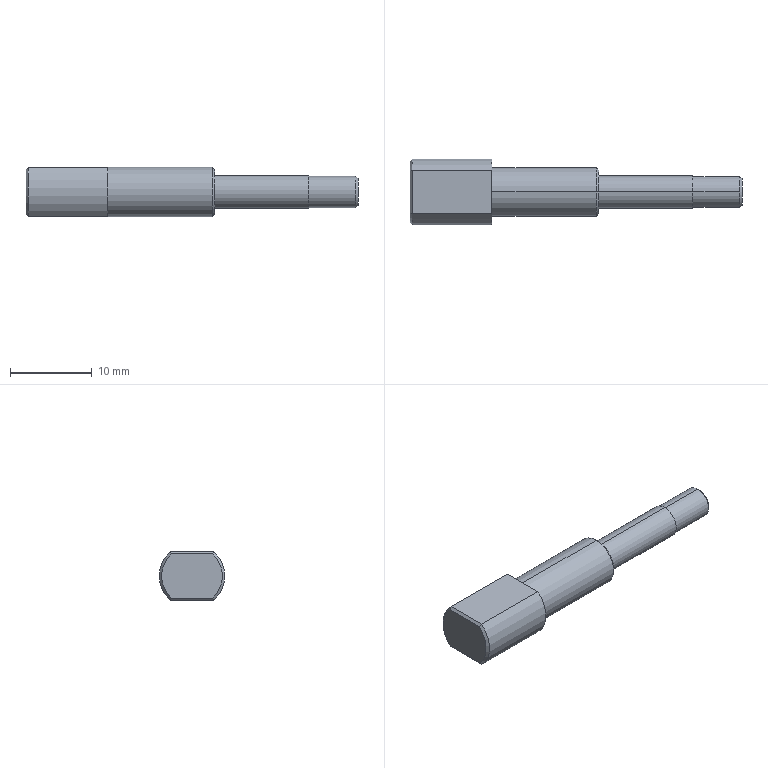Part | SolidWorks | features Chamfer 1, ICE 1, Revolution 1 | 1 solid | 24 faces | box 40.5 x 8 x 6 mm | volume 1008 mm3 | plane 10 | cylinder 8 | cone 6 | commonest cylinder face diameters 3.8 x2 4 x2 6 x2 8 x2
STEP:
#1=CARTESIAN_POINT('',(23.,0.,-2.7));
#2=VERTEX_POINT('',#1);
#3=CARTESIAN_POINT('',(23.,0.,2.7));
#4=VERTEX_POINT('',#3);
#5=CARTESIAN_POINT('',(23.,0.,0.));
#6=DIRECTION('',(1.,0.,0.));
#7=DIRECTION('',(0.,0.,1.));
#8=AXIS2_PLACEMENT_3D('',#5,#6,#7);
#9=CIRCLE('',#8,2.7);
#10=EDGE_CURVE('',#2,#4,#9,.T.);
#11=ORIENTED_EDGE('',*,*,#10,.F.);
#12=CARTESIAN_POINT('',(22.7,0.,-3.));
#13=VERTEX_POINT('',#12);
#14=CARTESIAN_POINT('',(22.7,0.,-3.));
#15=DIRECTION('',(-0.7071,0.,-0.7071));
#16=VECTOR('',#15,1000.);
#17=LINE('',#14,#16);
#18=EDGE_CURVE('',#2,#13,#17,.T.);
#19=ORIENTED_EDGE('',*,*,#18,.T.);
#20=CARTESIAN_POINT('',(22.7,0.,3.));
#21=VERTEX_POINT('',#20);
#22=CARTESIAN_POINT('',(22.7,0.,0.));
#23=DIRECTION('',(-1.,0.,0.));
#24=DIRECTION('',(0.,0.,1.));
#25=AXIS2_PLACEMENT_3D('',#22,#23,#24);
#26=CIRCLE('',#25,3.);
#27=EDGE_CURVE('',#21,#13,#26,.T.);
#28=ORIENTED_EDGE('',*,*,#27,.F.);
#29=CARTESIAN_POINT('',(22.7,0.,3.));
#30=DIRECTION('',(-0.7071,0.,0.7071));
#31=VECTOR('',#30,1000.);
#32=LINE('',#29,#31);
#33=EDGE_CURVE('',#4,#21,#32,.T.);
#34=ORIENTED_EDGE('',*,*,#33,.F.);
#35=EDGE_LOOP('',(#11,#19,#28,#34));
#36=FACE_OUTER_BOUND('',#35,.T.);
#37=CARTESIAN_POINT('',(22.7,0.,0.));
#38=DIRECTION('',(-1.,0.,0.));
#39=DIRECTION('',(0.,0.,1.));
#40=AXIS2_PLACEMENT_3D('',#37,#38,#39);
#41=CONICAL_SURFACE('',#40,3.,0.7854);
#42=ADVANCED_FACE('',(#36),#41,.T.);
#43=CARTESIAN_POINT('',(40.5,0.,-1.6));
#44=VERTEX_POINT('',#43);
#45=CARTESIAN_POINT('',(40.5,0.,1.6));
#46=VERTEX_POINT('',#45);
#47=CARTESIAN_POINT('',(40.5,0.,0.));
#48=DIRECTION('',(1.,0.,0.));
#49=DIRECTION('',(0.,0.,1.));
#50=AXIS2_PLACEMENT_3D('',#47,#48,#49);
#51=CIRCLE('',#50,1.6);
#52=EDGE_CURVE('',#44,#46,#51,.T.);
#53=ORIENTED_EDGE('',*,*,#52,.F.);
#54=CARTESIAN_POINT('',(40.2,0.,-1.9));
#55=VERTEX_POINT('',#54);
#56=CARTESIAN_POINT('',(40.2,0.,-1.9));
#57=DIRECTION('',(-0.7071,0.,-0.7071));
#58=VECTOR('',#57,1000.);
#59=LINE('',#56,#58);
#60=EDGE_CURVE('',#44,#55,#59,.T.);
#61=ORIENTED_EDGE('',*,*,#60,.T.);
#62=CARTESIAN_POINT('',(40.2,0.,1.9));
#63=VERTEX_POINT('',#62);
#64=CARTESIAN_POINT('',(40.2,0.,0.));
#65=DIRECTION('',(-1.,0.,0.));
#66=DIRECTION('',(0.,0.,1.));
#67=AXIS2_PLACEMENT_3D('',#64,#65,#66);
#68=CIRCLE('',#67,1.9);
#69=EDGE_CURVE('',#63,#55,#68,.T.);
#70=ORIENTED_EDGE('',*,*,#69,.F.);
#71=CARTESIAN_POINT('',(40.2,0.,1.9));
#72=DIRECTION('',(-0.7071,0.,0.7071));
#73=VECTOR('',#72,1000.);
#74=LINE('',#71,#73);
#75=EDGE_CURVE('',#46,#63,#74,.T.);
#76=ORIENTED_EDGE('',*,*,#75,.F.);
#77=EDGE_LOOP('',(#53,#61,#70,#76));
#78=FACE_OUTER_BOUND('',#77,.T.);
#79=CARTESIAN_POINT('',(40.2,0.,0.));
#80=DIRECTION('',(-1.,0.,0.));
#81=DIRECTION('',(0.,0.,1.));
#82=AXIS2_PLACEMENT_3D('',#79,#80,#81);
#83=CONICAL_SURFACE('',#82,1.9,0.7854);
#84=ADVANCED_FACE('',(#78),#83,.T.);
#85=ORIENTED_EDGE('',*,*,#69,.T.);
#86=CARTESIAN_POINT('',(34.5,0.,-1.9));
#87=VERTEX_POINT('',#86);
#88=CARTESIAN_POINT('',(0.,0.,-1.9));
#89=DIRECTION('',(-1.,0.,0.));
#90=VECTOR('',#89,1000.);
#91=LINE('',#88,#90);
#92=EDGE_CURVE('',#55,#87,#91,.T.);
#93=ORIENTED_EDGE('',*,*,#92,.T.);
#94=CARTESIAN_POINT('',(34.5,0.,1.9));
#95=VERTEX_POINT('',#94);
#96=CARTESIAN_POINT('',(34.5,0.,0.));
#97=DIRECTION('',(-1.,0.,0.));
#98=DIRECTION('',(0.,0.,1.));
#99=AXIS2_PLACEMENT_3D('',#96,#97,#98);
#100=CIRCLE('',#99,1.9);
#101=EDGE_CURVE('',#95,#87,#100,.T.);
#102=ORIENTED_EDGE('',*,*,#101,.F.);
#103=CARTESIAN_POINT('',(0.,0.,1.9));
#104=DIRECTION('',(-1.,0.,0.));
#105=VECTOR('',#104,1000.);
#106=LINE('',#103,#105);
#107=EDGE_CURVE('',#63,#95,#106,.T.);
#108=ORIENTED_EDGE('',*,*,#107,.F.);
#109=EDGE_LOOP('',(#85,#93,#102,#108));
#110=FACE_OUTER_BOUND('',#109,.T.);
#111=CARTESIAN_POINT('',(0.,0.,0.));
#112=DIRECTION('',(-1.,0.,0.));
#113=DIRECTION('',(0.,0.,1.));
#114=AXIS2_PLACEMENT_3D('',#111,#112,#113);
#115=CYLINDRICAL_SURFACE('',#114,1.9);
#116=ADVANCED_FACE('',(#110),#115,.T.);
#117=CARTESIAN_POINT('',(34.5,0.,2.));
#118=VERTEX_POINT('',#117);
#119=CARTESIAN_POINT('',(34.5,0.,-2.));
#120=VERTEX_POINT('',#119);
#121=CARTESIAN_POINT('',(34.5,0.,0.));
#122=DIRECTION('',(-1.,0.,0.));
#123=DIRECTION('',(0.,0.,1.));
#124=AXIS2_PLACEMENT_3D('',#121,#122,#123);
#125=CIRCLE('',#124,2.);
#126=EDGE_CURVE('',#118,#120,#125,.T.);
#127=ORIENTED_EDGE('',*,*,#126,.T.);
#128=CARTESIAN_POINT('',(23.,0.,-2.));
#129=VERTEX_POINT('',#128);
#130=CARTESIAN_POINT('',(0.,0.,-2.));
#131=DIRECTION('',(-1.,0.,0.));
#132=VECTOR('',#131,1000.);
#133=LINE('',#130,#132);
#134=EDGE_CURVE('',#120,#129,#133,.T.);
#135=ORIENTED_EDGE('',*,*,#134,.T.);
#136=CARTESIAN_POINT('',(23.,0.,2.));
#137=VERTEX_POINT('',#136);
#138=CARTESIAN_POINT('',(23.,0.,0.));
#139=DIRECTION('',(-1.,0.,0.));
#140=DIRECTION('',(0.,0.,1.));
#141=AXIS2_PLACEMENT_3D('',#138,#139,#140);
#142=CIRCLE('',#141,2.);
#143=EDGE_CURVE('',#137,#129,#142,.T.);
#144=ORIENTED_EDGE('',*,*,#143,.F.);
#145=CARTESIAN_POINT('',(0.,0.,2.));
#146=DIRECTION('',(-1.,0.,0.));
#147=VECTOR('',#146,1000.);
#148=LINE('',#145,#147);
#149=EDGE_CURVE('',#118,#137,#148,.T.);
#150=ORIENTED_EDGE('',*,*,#149,.F.);
#151=EDGE_LOOP('',(#127,#135,#144,#150));
#152=FACE_OUTER_BOUND('',#151,.T.);
#153=CARTESIAN_POINT('',(0.,0.,0.));
#154=DIRECTION('',(-1.,0.,0.));
#155=DIRECTION('',(0.,0.,1.));
#156=AXIS2_PLACEMENT_3D('',#153,#154,#155);
#157=CYLINDRICAL_SURFACE('',#156,2.);
#158=ADVANCED_FACE('',(#152),#157,.T.);
#159=ORIENTED_EDGE('',*,*,#27,.T.);
#160=CARTESIAN_POINT('',(10.,0.,-3.));
#161=VERTEX_POINT('',#160);
#162=CARTESIAN_POINT('',(0.,0.,-3.));
#163=DIRECTION('',(-1.,0.,0.));
#164=VECTOR('',#163,1000.);
#165=LINE('',#162,#164);
#166=EDGE_CURVE('',#13,#161,#165,.T.);
#167=ORIENTED_EDGE('',*,*,#166,.T.);
#168=CARTESIAN_POINT('',(10.,0.,3.));
#169=VERTEX_POINT('',#168);
#170=CARTESIAN_POINT('',(10.,0.,0.));
#171=DIRECTION('',(-1.,0.,0.));
#172=DIRECTION('',(0.,0.,1.));
#173=AXIS2_PLACEMENT_3D('',#170,#171,#172);
#174=CIRCLE('',#173,3.);
#175=EDGE_CURVE('',#169,#161,#174,.T.);
#176=ORIENTED_EDGE('',*,*,#175,.F.);
#177=CARTESIAN_POINT('',(0.,0.,3.));
#178=DIRECTION('',(-1.,0.,0.));
#179=VECTOR('',#178,1000.);
#180=LINE('',#177,#179);
#181=EDGE_CURVE('',#21,#169,#180,.T.);
#182=ORIENTED_EDGE('',*,*,#181,.F.);
#183=EDGE_LOOP('',(#159,#167,#176,#182));
#184=FACE_OUTER_BOUND('',#183,.T.);
#185=CARTESIAN_POINT('',(0.,0.,0.));
#186=DIRECTION('',(-1.,0.,0.));
#187=DIRECTION('',(0.,0.,1.));
#188=AXIS2_PLACEMENT_3D('',#185,#186,#187);
#189=CYLINDRICAL_SURFACE('',#188,3.);
#190=ADVANCED_FACE('',(#184),#189,.T.);
#191=CARTESIAN_POINT('',(0.3,2.646,-3.));
#192=VERTEX_POINT('',#191);
#193=CARTESIAN_POINT('',(10.,2.646,-3.));
#194=VERTEX_POINT('',#193);
#195=CARTESIAN_POINT('',(0.,2.646,-3.));
#196=DIRECTION('',(1.,0.,0.));
#197=VECTOR('',#196,1000.);
#198=LINE('',#195,#197);
#199=EDGE_CURVE('',#192,#194,#198,.T.);
#200=ORIENTED_EDGE('',*,*,#199,.F.);
#201=CARTESIAN_POINT('',(0.3,2.646,3.));
#202=VERTEX_POINT('',#201);
#203=CARTESIAN_POINT('',(0.3,0.,0.));
#204=DIRECTION('',(1.,0.,0.));
#205=DIRECTION('',(0.,0.,-1.));
#206=AXIS2_PLACEMENT_3D('',#203,#204,#205);
#207=CIRCLE('',#206,4.);
#208=EDGE_CURVE('',#192,#202,#207,.T.);
#209=ORIENTED_EDGE('',*,*,#208,.T.);
#210=CARTESIAN_POINT('',(10.,2.646,3.));
#211=VERTEX_POINT('',#210);
#212=CARTESIAN_POINT('',(0.,2.646,3.));
#213=DIRECTION('',(-1.,0.,0.));
#214=VECTOR('',#213,1000.);
#215=LINE('',#212,#214);
#216=EDGE_CURVE('',#211,#202,#215,.T.);
#217=ORIENTED_EDGE('',*,*,#216,.F.);
#218=CARTESIAN_POINT('',(10.,0.,0.));
#219=DIRECTION('',(-1.,0.,0.));
#220=DIRECTION('',(0.,0.,1.));
#221=AXIS2_PLACEMENT_3D('',#218,#219,#220);
#222=CIRCLE('',#221,4.);
#223=EDGE_CURVE('',#211,#194,#222,.T.);
#224=ORIENTED_EDGE('',*,*,#223,.T.);
#225=EDGE_LOOP('',(#200,#209,#217,#224));
#226=FACE_OUTER_BOUND('',#225,.T.);
#227=CARTESIAN_POINT('',(0.,0.,0.));
#228=DIRECTION('',(-1.,0.,0.));
#229=DIRECTION('',(0.,0.,1.));
#230=AXIS2_PLACEMENT_3D('',#227,#228,#229);
#231=CYLINDRICAL_SURFACE('',#230,4.);
#232=ADVANCED_FACE('',(#226),#231,.T.);
#233=CARTESIAN_POINT('',(10.,-2.646,-3.));
#234=VERTEX_POINT('',#233);
#235=CARTESIAN_POINT('',(10.,-2.646,3.));
#236=VERTEX_POINT('',#235);
#237=CARTESIAN_POINT('',(10.,0.,0.));
#238=DIRECTION('',(-1.,0.,0.));
#239=DIRECTION('',(0.,0.,1.));
#240=AXIS2_PLACEMENT_3D('',#237,#238,#239);
#241=CIRCLE('',#240,4.);
#242=EDGE_CURVE('',#234,#236,#241,.T.);
#243=ORIENTED_EDGE('',*,*,#242,.F.);
#244=CARTESIAN_POINT('',(10.,4.651,-3.));
#245=DIRECTION('',(0.,-1.,0.));
#246=VECTOR('',#245,1000.);
#247=LINE('',#244,#246);
#248=EDGE_CURVE('',#161,#234,#247,.T.);
#249=ORIENTED_EDGE('',*,*,#248,.F.);
#250=CARTESIAN_POINT('',(10.,0.,0.));
#251=DIRECTION('',(-1.,0.,0.));
#252=DIRECTION('',(0.,0.,1.));
#253=AXIS2_PLACEMENT_3D('',#250,#251,#252);
#254=CIRCLE('',#253,3.);
#255=EDGE_CURVE('',#161,#169,#254,.T.);
#256=ORIENTED_EDGE('',*,*,#255,.T.);
#257=CARTESIAN_POINT('',(10.,4.254,3.));
#258=DIRECTION('',(0.,1.,0.));
#259=VECTOR('',#258,1000.);
#260=LINE('',#257,#259);
#261=EDGE_CURVE('',#236,#169,#260,.T.);
#262=ORIENTED_EDGE('',*,*,#261,.F.);
#263=EDGE_LOOP('',(#243,#249,#256,#262));
#264=FACE_OUTER_BOUND('',#263,.T.);
#265=CARTESIAN_POINT('',(10.,4.,0.));
#266=DIRECTION('',(-1.,0.,0.));
#267=DIRECTION('',(0.,0.,1.));
#268=AXIS2_PLACEMENT_3D('',#265,#266,#267);
#269=PLANE('',#268);
#270=ADVANCED_FACE('',(#264),#269,.F.);
#271=CARTESIAN_POINT('',(0.,-2.53,-2.7));
#272=VERTEX_POINT('',#271);
#273=CARTESIAN_POINT('',(0.,-2.53,2.7));
#274=VERTEX_POINT('',#273);
#275=CARTESIAN_POINT('',(0.,0.,0.));
#276=DIRECTION('',(-1.,0.,0.));
#277=DIRECTION('',(0.,0.,-1.));
#278=AXIS2_PLACEMENT_3D('',#275,#276,#277);
#279=CIRCLE('',#278,3.7);
#280=EDGE_CURVE('',#272,#274,#279,.T.);
#281=ORIENTED_EDGE('',*,*,#280,.T.);
#282=CARTESIAN_POINT('',(0.,2.53,2.7));
#283=VERTEX_POINT('',#282);
#284=CARTESIAN_POINT('',(0.,0.,2.7));
#285=DIRECTION('',(0.,1.,0.));
#286=VECTOR('',#285,1000.);
#287=LINE('',#284,#286);
#288=EDGE_CURVE('',#274,#283,#287,.T.);
#289=ORIENTED_EDGE('',*,*,#288,.T.);
#290=CARTESIAN_POINT('',(0.,2.53,-2.7));
#291=VERTEX_POINT('',#290);
#292=CARTESIAN_POINT('',(0.,0.,0.));
#293=DIRECTION('',(-1.,0.,0.));
#294=DIRECTION('',(0.,0.,-1.));
#295=AXIS2_PLACEMENT_3D('',#292,#293,#294);
#296=CIRCLE('',#295,3.7);
#297=EDGE_CURVE('',#283,#291,#296,.T.);
#298=ORIENTED_EDGE('',*,*,#297,.T.);
#299=CARTESIAN_POINT('',(0.,0.,-2.7));
#300=DIRECTION('',(0.,-1.,0.));
#301=VECTOR('',#300,1000.);
#302=LINE('',#299,#301);
#303=EDGE_CURVE('',#291,#272,#302,.T.);
#304=ORIENTED_EDGE('',*,*,#303,.T.);
#305=EDGE_LOOP('',(#281,#289,#298,#304));
#306=FACE_OUTER_BOUND('',#305,.T.);
#307=CARTESIAN_POINT('',(0.,0.,0.));
#308=DIRECTION('',(1.,0.,0.));
#309=DIRECTION('',(0.,0.,-1.));
#310=AXIS2_PLACEMENT_3D('',#307,#308,#309);
#311=PLANE('',#310);
#312=ADVANCED_FACE('',(#306),#311,.F.);
#313=CARTESIAN_POINT('',(0.3,-2.646,3.));
#314=VERTEX_POINT('',#313);
#315=CARTESIAN_POINT('',(0.,-2.646,3.));
#316=DIRECTION('',(1.,0.,0.));
#317=VECTOR('',#316,1000.);
#318=LINE('',#315,#317);
#319=EDGE_CURVE('',#314,#236,#318,.T.);
#320=ORIENTED_EDGE('',*,*,#319,.F.);
#321=CARTESIAN_POINT('',(0.3,-2.646,-3.));
#322=VERTEX_POINT('',#321);
#323=CARTESIAN_POINT('',(0.3,0.,0.));
#324=DIRECTION('',(1.,0.,0.));
#325=DIRECTION('',(0.,0.,-1.));
#326=AXIS2_PLACEMENT_3D('',#323,#324,#325);
#327=CIRCLE('',#326,4.);
#328=EDGE_CURVE('',#314,#322,#327,.T.);
#329=ORIENTED_EDGE('',*,*,#328,.T.);
#330=CARTESIAN_POINT('',(0.,-2.646,-3.));
#331=DIRECTION('',(-1.,0.,0.));
#332=VECTOR('',#331,1000.);
#333=LINE('',#330,#332);
#334=EDGE_CURVE('',#234,#322,#333,.T.);
#335=ORIENTED_EDGE('',*,*,#334,.F.);
#336=ORIENTED_EDGE('',*,*,#242,.T.);
#337=EDGE_LOOP('',(#320,#329,#335,#336));
#338=FACE_OUTER_BOUND('',#337,.T.);
#339=CARTESIAN_POINT('',(0.,0.,0.));
#340=DIRECTION('',(-1.,0.,0.));
#341=DIRECTION('',(0.,0.,1.));
#342=AXIS2_PLACEMENT_3D('',#339,#340,#341);
#343=CYLINDRICAL_SURFACE('',#342,4.);
#344=ADVANCED_FACE('',(#338),#343,.T.);
#345=ORIENTED_EDGE('',*,*,#175,.T.);
#346=CARTESIAN_POINT('',(10.,4.651,-3.));
#347=DIRECTION('',(0.,-1.,0.));
#348=VECTOR('',#347,1000.);
#349=LINE('',#346,#348);
#350=EDGE_CURVE('',#194,#161,#349,.T.);
#351=ORIENTED_EDGE('',*,*,#350,.F.);
#352=ORIENTED_EDGE('',*,*,#223,.F.);
#353=CARTESIAN_POINT('',(10.,4.254,3.));
#354=DIRECTION('',(0.,1.,0.));
#355=VECTOR('',#354,1000.);
#356=LINE('',#353,#355);
#357=EDGE_CURVE('',#169,#211,#356,.T.);
#358=ORIENTED_EDGE('',*,*,#357,.F.);
#359=EDGE_LOOP('',(#345,#351,#352,#358));
#360=FACE_OUTER_BOUND('',#359,.T.);
#361=CARTESIAN_POINT('',(10.,4.,0.));
#362=DIRECTION('',(-1.,0.,0.));
#363=DIRECTION('',(0.,0.,1.));
#364=AXIS2_PLACEMENT_3D('',#361,#362,#363);
#365=PLANE('',#364);
#366=ADVANCED_FACE('',(#360),#365,.F.);
#367=ORIENTED_EDGE('',*,*,#166,.F.);
#368=CARTESIAN_POINT('',(22.7,0.,0.));
#369=DIRECTION('',(-1.,0.,0.));
#370=DIRECTION('',(0.,0.,1.));
#371=AXIS2_PLACEMENT_3D('',#368,#369,#370);
#372=CIRCLE('',#371,3.);
#373=EDGE_CURVE('',#13,#21,#372,.T.);
#374=ORIENTED_EDGE('',*,*,#373,.T.);
#375=ORIENTED_EDGE('',*,*,#181,.T.);
#376=ORIENTED_EDGE('',*,*,#255,.F.);
#377=EDGE_LOOP('',(#367,#374,#375,#376));
#378=FACE_OUTER_BOUND('',#377,.T.);
#379=CARTESIAN_POINT('',(0.,0.,0.));
#380=DIRECTION('',(-1.,0.,0.));
#381=DIRECTION('',(0.,0.,1.));
#382=AXIS2_PLACEMENT_3D('',#379,#380,#381);
#383=CYLINDRICAL_SURFACE('',#382,3.);
#384=ADVANCED_FACE('',(#378),#383,.T.);
#385=CARTESIAN_POINT('',(23.,0.,0.));
#386=DIRECTION('',(1.,0.,0.));
#387=DIRECTION('',(0.,0.,1.));
#388=AXIS2_PLACEMENT_3D('',#385,#386,#387);
#389=CIRCLE('',#388,2.7);
#390=EDGE_CURVE('',#4,#2,#389,.T.);
#391=ORIENTED_EDGE('',*,*,#390,.T.);
#392=ORIENTED_EDGE('',*,*,#10,.T.);
#393=EDGE_LOOP('',(#391,#392));
#394=FACE_OUTER_BOUND('',#393,.T.);
#395=ORIENTED_EDGE('',*,*,#143,.T.);
#396=CARTESIAN_POINT('',(23.,0.,0.));
#397=DIRECTION('',(-1.,0.,0.));
#398=DIRECTION('',(0.,0.,1.));
#399=AXIS2_PLACEMENT_3D('',#396,#397,#398);
#400=CIRCLE('',#399,2.);
#401=EDGE_CURVE('',#129,#137,#400,.T.);
#402=ORIENTED_EDGE('',*,*,#401,.T.);
#403=EDGE_LOOP('',(#395,#402));
#404=FACE_BOUND('',#403,.T.);
#405=CARTESIAN_POINT('',(23.,3.,0.));
#406=DIRECTION('',(-1.,0.,0.));
#407=DIRECTION('',(0.,0.,1.));
#408=AXIS2_PLACEMENT_3D('',#405,#406,#407);
#409=PLANE('',#408);
#410=ADVANCED_FACE('',(#394,#404),#409,.F.);
#411=ORIENTED_EDGE('',*,*,#134,.F.);
#412=CARTESIAN_POINT('',(34.5,0.,0.));
#413=DIRECTION('',(-1.,0.,0.));
#414=DIRECTION('',(0.,0.,1.));
#415=AXIS2_PLACEMENT_3D('',#412,#413,#414);
#416=CIRCLE('',#415,2.);
#417=EDGE_CURVE('',#120,#118,#416,.T.);
#418=ORIENTED_EDGE('',*,*,#417,.T.);
#419=ORIENTED_EDGE('',*,*,#149,.T.);
#420=ORIENTED_EDGE('',*,*,#401,.F.);
#421=EDGE_LOOP('',(#411,#418,#419,#420));
#422=FACE_OUTER_BOUND('',#421,.T.);
#423=CARTESIAN_POINT('',(0.,0.,0.));
#424=DIRECTION('',(-1.,0.,0.));
#425=DIRECTION('',(0.,0.,1.));
#426=AXIS2_PLACEMENT_3D('',#423,#424,#425);
#427=CYLINDRICAL_SURFACE('',#426,2.);
#428=ADVANCED_FACE('',(#422),#427,.T.);
#429=ORIENTED_EDGE('',*,*,#126,.F.);
#430=ORIENTED_EDGE('',*,*,#417,.F.);
#431=EDGE_LOOP('',(#429,#430));
#432=FACE_OUTER_BOUND('',#431,.T.);
#433=ORIENTED_EDGE('',*,*,#101,.T.);
#434=CARTESIAN_POINT('',(34.5,0.,0.));
#435=DIRECTION('',(-1.,0.,0.));
#436=DIRECTION('',(0.,0.,1.));
#437=AXIS2_PLACEMENT_3D('',#434,#435,#436);
#438=CIRCLE('',#437,1.9);
#439=EDGE_CURVE('',#87,#95,#438,.T.);
#440=ORIENTED_EDGE('',*,*,#439,.T.);
#441=EDGE_LOOP('',(#433,#440));
#442=FACE_BOUND('',#441,.T.);
#443=CARTESIAN_POINT('',(34.5,2.,0.));
#444=DIRECTION('',(-1.,0.,0.));
#445=DIRECTION('',(0.,0.,1.));
#446=AXIS2_PLACEMENT_3D('',#443,#444,#445);
#447=PLANE('',#446);
#448=ADVANCED_FACE('',(#432,#442),#447,.F.);
#449=ORIENTED_EDGE('',*,*,#92,.F.);
#450=CARTESIAN_POINT('',(40.2,0.,0.));
#451=DIRECTION('',(-1.,0.,0.));
#452=DIRECTION('',(0.,0.,1.));
#453=AXIS2_PLACEMENT_3D('',#450,#451,#452);
#454=CIRCLE('',#453,1.9);
#455=EDGE_CURVE('',#55,#63,#454,.T.);
#456=ORIENTED_EDGE('',*,*,#455,.T.);
#457=ORIENTED_EDGE('',*,*,#107,.T.);
#458=ORIENTED_EDGE('',*,*,#439,.F.);
#459=EDGE_LOOP('',(#449,#456,#457,#458));
#460=FACE_OUTER_BOUND('',#459,.T.);
#461=CARTESIAN_POINT('',(0.,0.,0.));
#462=DIRECTION('',(-1.,0.,0.));
#463=DIRECTION('',(0.,0.,1.));
#464=AXIS2_PLACEMENT_3D('',#461,#462,#463);
#465=CYLINDRICAL_SURFACE('',#464,1.9);
#466=ADVANCED_FACE('',(#460),#465,.T.);
#467=CARTESIAN_POINT('',(40.5,0.,0.));
#468=DIRECTION('',(1.,0.,0.));
#469=DIRECTION('',(0.,0.,1.));
#470=AXIS2_PLACEMENT_3D('',#467,#468,#469);
#471=CIRCLE('',#470,1.6);
#472=EDGE_CURVE('',#46,#44,#471,.T.);
#473=ORIENTED_EDGE('',*,*,#472,.T.);
#474=ORIENTED_EDGE('',*,*,#52,.T.);
#475=EDGE_LOOP('',(#473,#474));
#476=FACE_OUTER_BOUND('',#475,.T.);
#477=CARTESIAN_POINT('',(40.5,1.9,0.));
#478=DIRECTION('',(-1.,0.,0.));
#479=DIRECTION('',(0.,0.,1.));
#480=AXIS2_PLACEMENT_3D('',#477,#478,#479);
#481=PLANE('',#480);
#482=ADVANCED_FACE('',(#476),#481,.F.);
#483=ORIENTED_EDGE('',*,*,#216,.T.);
#484=CARTESIAN_POINT('',(0.3,4.254,3.));
#485=DIRECTION('',(0.,-1.,0.));
#486=VECTOR('',#485,1000.);
#487=LINE('',#484,#486);
#488=EDGE_CURVE('',#202,#314,#487,.T.);
#489=ORIENTED_EDGE('',*,*,#488,.T.);
#490=ORIENTED_EDGE('',*,*,#319,.T.);
#491=ORIENTED_EDGE('',*,*,#261,.T.);
#492=ORIENTED_EDGE('',*,*,#357,.T.);
#493=EDGE_LOOP('',(#483,#489,#490,#491,#492));
#494=FACE_OUTER_BOUND('',#493,.T.);
#495=CARTESIAN_POINT('',(40.501,4.254,3.));
#496=DIRECTION('',(0.,0.,-1.));
#497=DIRECTION('',(0.,1.,0.));
#498=AXIS2_PLACEMENT_3D('',#495,#496,#497);
#499=PLANE('',#498);
#500=ADVANCED_FACE('',(#494),#499,.F.);
#501=ORIENTED_EDGE('',*,*,#334,.T.);
#502=CARTESIAN_POINT('',(0.3,4.651,-3.));
#503=DIRECTION('',(0.,1.,0.));
#504=VECTOR('',#503,1000.);
#505=LINE('',#502,#504);
#506=EDGE_CURVE('',#322,#192,#505,.T.);
#507=ORIENTED_EDGE('',*,*,#506,.T.);
#508=ORIENTED_EDGE('',*,*,#199,.T.);
#509=ORIENTED_EDGE('',*,*,#350,.T.);
#510=ORIENTED_EDGE('',*,*,#248,.T.);
#511=EDGE_LOOP('',(#501,#507,#508,#509,#510));
#512=FACE_OUTER_BOUND('',#511,.T.);
#513=CARTESIAN_POINT('',(40.501,4.651,-3.));
#514=DIRECTION('',(0.,0.,1.));
#515=DIRECTION('',(1.,0.,0.));
#516=AXIS2_PLACEMENT_3D('',#513,#514,#515);
#517=PLANE('',#516);
#518=ADVANCED_FACE('',(#512),#517,.F.);
#519=CARTESIAN_POINT('',(0.,-2.53,-2.7));
#520=CARTESIAN_POINT('',(0.09984,-2.569,-2.8));
#521=CARTESIAN_POINT('',(0.1998,-2.608,-2.9));
#522=CARTESIAN_POINT('',(0.3,-2.646,-3.));
#523=B_SPLINE_CURVE_WITH_KNOTS('',3,(#519,#520,#521,#522),.UNSPECIFIED.,.F.,.F.,(4,4),(0.,0.0004398),.UNSPECIFIED.);
#524=EDGE_CURVE('',#272,#322,#523,.T.);
#525=ORIENTED_EDGE('',*,*,#524,.F.);
#526=ORIENTED_EDGE('',*,*,#303,.F.);
#527=CARTESIAN_POINT('',(0.3,2.646,-3.));
#528=CARTESIAN_POINT('',(0.1998,2.608,-2.9));
#529=CARTESIAN_POINT('',(0.09984,2.569,-2.8));
#530=CARTESIAN_POINT('',(0.,2.53,-2.7));
#531=B_SPLINE_CURVE_WITH_KNOTS('',3,(#527,#528,#529,#530),.UNSPECIFIED.,.F.,.F.,(4,4),(0.,0.0004398),.UNSPECIFIED.);
#532=EDGE_CURVE('',#192,#291,#531,.T.);
#533=ORIENTED_EDGE('',*,*,#532,.F.);
#534=ORIENTED_EDGE('',*,*,#506,.F.);
#535=EDGE_LOOP('',(#525,#526,#533,#534));
#536=FACE_OUTER_BOUND('',#535,.T.);
#537=CARTESIAN_POINT('',(0.3,4.651,-3.));
#538=DIRECTION('',(0.7071,0.,0.7071));
#539=DIRECTION('',(0.,1.,0.));
#540=AXIS2_PLACEMENT_3D('',#537,#538,#539);
#541=PLANE('',#540);
#542=ADVANCED_FACE('',(#536),#541,.F.);
#543=ORIENTED_EDGE('',*,*,#532,.T.);
#544=ORIENTED_EDGE('',*,*,#297,.F.);
#545=CARTESIAN_POINT('',(0.3,2.646,3.));
#546=CARTESIAN_POINT('',(0.1998,2.608,2.9));
#547=CARTESIAN_POINT('',(0.09984,2.569,2.8));
#548=CARTESIAN_POINT('',(0.,2.53,2.7));
#549=B_SPLINE_CURVE_WITH_KNOTS('',3,(#545,#546,#547,#548),.UNSPECIFIED.,.F.,.F.,(4,4),(0.,0.0004398),.UNSPECIFIED.);
#550=EDGE_CURVE('',#202,#283,#549,.T.);
#551=ORIENTED_EDGE('',*,*,#550,.F.);
#552=ORIENTED_EDGE('',*,*,#208,.F.);
#553=EDGE_LOOP('',(#543,#544,#551,#552));
#554=FACE_OUTER_BOUND('',#553,.T.);
#555=CARTESIAN_POINT('',(0.,0.,0.));
#556=DIRECTION('',(1.,0.,0.));
#557=DIRECTION('',(0.,0.,-1.));
#558=AXIS2_PLACEMENT_3D('',#555,#556,#557);
#559=CONICAL_SURFACE('',#558,3.7,0.7854);
#560=ADVANCED_FACE('',(#554),#559,.T.);
#561=ORIENTED_EDGE('',*,*,#524,.T.);
#562=ORIENTED_EDGE('',*,*,#328,.F.);
#563=CARTESIAN_POINT('',(0.,-2.53,2.7));
#564=CARTESIAN_POINT('',(0.09984,-2.569,2.8));
#565=CARTESIAN_POINT('',(0.1998,-2.608,2.9));
#566=CARTESIAN_POINT('',(0.3,-2.646,3.));
#567=B_SPLINE_CURVE_WITH_KNOTS('',3,(#563,#564,#565,#566),.UNSPECIFIED.,.F.,.F.,(4,4),(0.,0.0004398),.UNSPECIFIED.);
#568=EDGE_CURVE('',#274,#314,#567,.T.);
#569=ORIENTED_EDGE('',*,*,#568,.F.);
#570=ORIENTED_EDGE('',*,*,#280,.F.);
#571=EDGE_LOOP('',(#561,#562,#569,#570));
#572=FACE_OUTER_BOUND('',#571,.T.);
#573=CARTESIAN_POINT('',(0.,0.,0.));
#574=DIRECTION('',(1.,0.,0.));
#575=DIRECTION('',(0.,0.,-1.));
#576=AXIS2_PLACEMENT_3D('',#573,#574,#575);
#577=CONICAL_SURFACE('',#576,3.7,0.7854);
#578=ADVANCED_FACE('',(#572),#577,.T.);
#579=ORIENTED_EDGE('',*,*,#550,.T.);
#580=ORIENTED_EDGE('',*,*,#288,.F.);
#581=ORIENTED_EDGE('',*,*,#568,.T.);
#582=ORIENTED_EDGE('',*,*,#488,.F.);
#583=EDGE_LOOP('',(#579,#580,#581,#582));
#584=FACE_OUTER_BOUND('',#583,.T.);
#585=CARTESIAN_POINT('',(0.3,4.254,3.));
#586=DIRECTION('',(0.7071,0.,-0.7071));
#587=DIRECTION('',(0.,-1.,0.));
#588=AXIS2_PLACEMENT_3D('',#585,#586,#587);
#589=PLANE('',#588);
#590=ADVANCED_FACE('',(#584),#589,.F.);
#591=ORIENTED_EDGE('',*,*,#60,.F.);
#592=ORIENTED_EDGE('',*,*,#472,.F.);
#593=ORIENTED_EDGE('',*,*,#75,.T.);
#594=ORIENTED_EDGE('',*,*,#455,.F.);
#595=EDGE_LOOP('',(#591,#592,#593,#594));
#596=FACE_OUTER_BOUND('',#595,.T.);
#597=CARTESIAN_POINT('',(40.2,0.,0.));
#598=DIRECTION('',(-1.,0.,0.));
#599=DIRECTION('',(0.,0.,1.));
#600=AXIS2_PLACEMENT_3D('',#597,#598,#599);
#601=CONICAL_SURFACE('',#600,1.9,0.7854);
#602=ADVANCED_FACE('',(#596),#601,.T.);
#603=ORIENTED_EDGE('',*,*,#18,.F.);
#604=ORIENTED_EDGE('',*,*,#390,.F.);
#605=ORIENTED_EDGE('',*,*,#33,.T.);
#606=ORIENTED_EDGE('',*,*,#373,.F.);
#607=EDGE_LOOP('',(#603,#604,#605,#606));
#608=FACE_OUTER_BOUND('',#607,.T.);
#609=CARTESIAN_POINT('',(22.7,0.,0.));
#610=DIRECTION('',(-1.,0.,0.));
#611=DIRECTION('',(0.,0.,1.));
#612=AXIS2_PLACEMENT_3D('',#609,#610,#611);
#613=CONICAL_SURFACE('',#612,3.,0.7854);
#614=ADVANCED_FACE('',(#608),#613,.T.);
#615=CLOSED_SHELL('',(#42,#84,#116,#158,#190,#232,#270,#312,#344,#366,#384,#410,#428,#448,#466,#482,#500,#518,#542,#560,#578,#590,#602,#614));
#616=MANIFOLD_SOLID_BREP('',#615);
#617=CARTESIAN_POINT('',(0.,0.,0.));
#618=DIRECTION('',(0.,0.,1.));
#619=DIRECTION('',(1.,0.,0.));
#620=AXIS2_PLACEMENT_3D('',#617,#618,#619);
#621=(LENGTH_UNIT()NAMED_UNIT(*)SI_UNIT(.MILLI.,.METRE.));
#622=UNCERTAINTY_MEASURE_WITH_UNIT(LENGTH_MEASURE(0.00001),#621,'','');
#623=(NAMED_UNIT(*)PLANE_ANGLE_UNIT()SI_UNIT($,.RADIAN.));
#624=(NAMED_UNIT(*)SI_UNIT($,.STERADIAN.)SOLID_ANGLE_UNIT());
#625=(GEOMETRIC_REPRESENTATION_CONTEXT(3)GLOBAL_UNCERTAINTY_ASSIGNED_CONTEXT((#622))GLOBAL_UNIT_ASSIGNED_CONTEXT((#621,#623,#624))REPRESENTATION_CONTEXT('',''));
#626=ADVANCED_BREP_SHAPE_REPRESENTATION('',(#616,#620),#625);